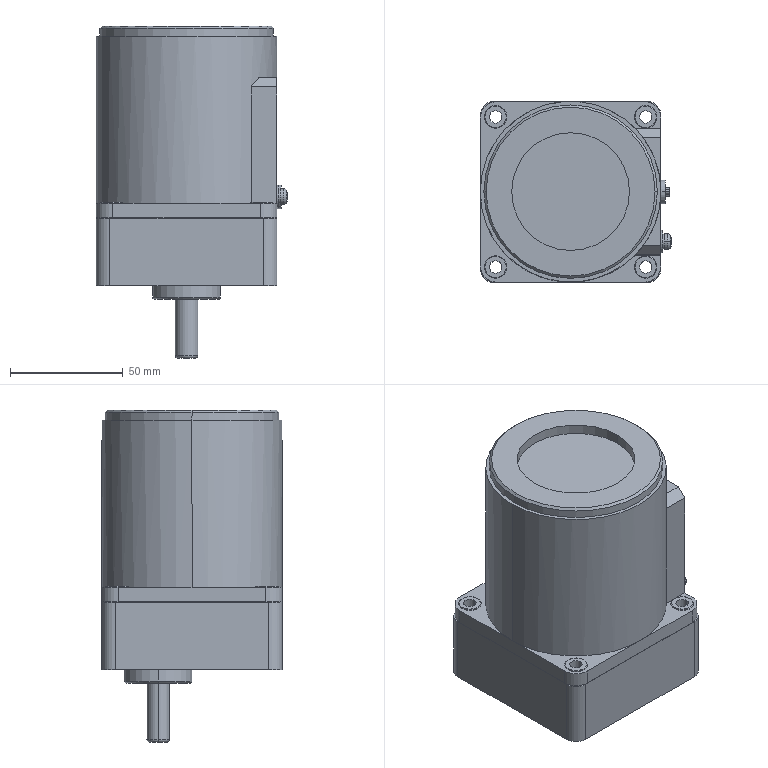Part | STEP file | Guide wheel mechanism revised.sldasm-Part-77 | 1 solid | 123 faces | box 84.773 x 80 x 147 mm | volume 629589 mm3 | plane 53 | cylinder 52 | torus 14 | sphere 2 | cone 2 | commonest cylinder face diameters 10 x12 5.5 x8 2 x6 12 x4 12.6 x4 14.6 x4